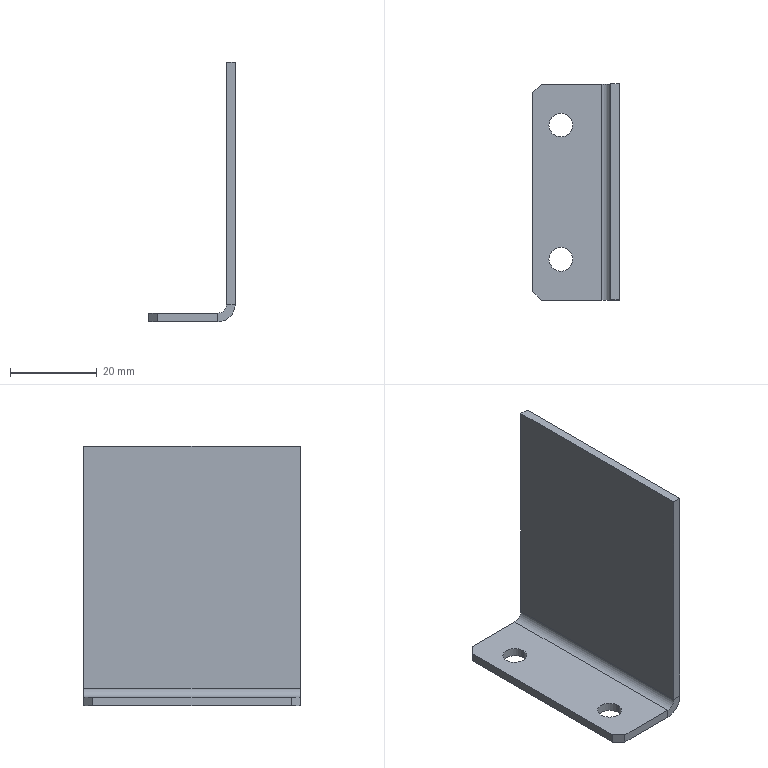Part | STEP file | Cable fixing bracket 1001 | 1 solid | 20 faces | box 20 x 50 x 60 mm | volume 7568 mm3 | plane 14 | cylinder 6 | commonest cylinder face diameters 5.5 x4 4 x1 8 x1
STEP:
#1=CARTESIAN_POINT('',(0.,0.,0.));
#2=DIRECTION('',(0.,0.,1.));
#3=DIRECTION('',(1.,0.,0.));
#4=AXIS2_PLACEMENT_3D('',#1,#2,#3);
#5=CARTESIAN_POINT('',(-16.25,15.5,2.));
#6=VERTEX_POINT('',#5);
#7=CARTESIAN_POINT('',(-16.25,15.5,0.));
#8=VERTEX_POINT('',#7);
#9=CARTESIAN_POINT('',(-16.25,15.5,60.));
#10=DIRECTION('',(0.,0.,-1.));
#11=VECTOR('',#10,1.);
#12=LINE('',#9,#11);
#13=CARTESIAN_POINT('',(-13.5,15.5,60.));
#14=DIRECTION('',(0.,0.,-1.));
#15=DIRECTION('',(-1.,0.,0.));
#16=AXIS2_PLACEMENT_3D('',#13,#14,#15);
#17=CYLINDRICAL_SURFACE('',#16,2.75);
#18=CARTESIAN_POINT('',(6.283,0.));
#19=DIRECTION('',(0.,1.));
#20=VECTOR('',#19,1.);
#21=LINE('',#18,#20);
#22=(GEOMETRIC_REPRESENTATION_CONTEXT(2)PARAMETRIC_REPRESENTATION_CONTEXT()REPRESENTATION_CONTEXT('',''));
#23=DEFINITIONAL_REPRESENTATION('',(#21),#22);
#24=PCURVE('',#17,#23);
#25=CARTESIAN_POINT('',(-13.5,15.5,60.));
#26=DIRECTION('',(0.,0.,-1.));
#27=DIRECTION('',(-1.,0.,0.));
#28=AXIS2_PLACEMENT_3D('',#25,#26,#27);
#29=CYLINDRICAL_SURFACE('',#28,2.75);
#30=CARTESIAN_POINT('',(0.,0.));
#31=DIRECTION('',(0.,1.));
#32=VECTOR('',#31,1.);
#33=LINE('',#30,#32);
#34=(GEOMETRIC_REPRESENTATION_CONTEXT(2)PARAMETRIC_REPRESENTATION_CONTEXT()REPRESENTATION_CONTEXT('',''));
#35=DEFINITIONAL_REPRESENTATION('',(#33),#34);
#36=PCURVE('',#29,#35);
#37=SURFACE_CURVE('',#12,(#24,#36),.PCURVE_S1.);
#38=EDGE_CURVE('',#6,#8,#37,.T.);
#39=ORIENTED_EDGE('',*,*,#38,.T.);
#40=CARTESIAN_POINT('',(-10.75,15.5,0.));
#41=VERTEX_POINT('',#40);
#42=CARTESIAN_POINT('',(-13.5,15.5,0.));
#43=DIRECTION('',(0.,0.,-1.));
#44=DIRECTION('',(-1.,0.,0.));
#45=AXIS2_PLACEMENT_3D('',#42,#43,#44);
#46=CIRCLE('',#45,2.75);
#47=CARTESIAN_POINT('',(0.,60.));
#48=DIRECTION('',(1.,0.));
#49=VECTOR('',#48,1.);
#50=LINE('',#47,#49);
#51=(GEOMETRIC_REPRESENTATION_CONTEXT(2)PARAMETRIC_REPRESENTATION_CONTEXT()REPRESENTATION_CONTEXT('',''));
#52=DEFINITIONAL_REPRESENTATION('',(#50),#51);
#53=PCURVE('',#17,#52);
#54=CARTESIAN_POINT('',(-20.,25.,0.));
#55=DIRECTION('',(0.,0.,-1.));
#56=DIRECTION('',(-1.,0.,0.));
#57=AXIS2_PLACEMENT_3D('',#54,#55,#56);
#58=PLANE('',#57);
#59=CARTESIAN_POINT('',(-6.5,-9.5));
#60=DIRECTION('',(1.,0.));
#61=AXIS2_PLACEMENT_2D('',#59,#60);
#62=CIRCLE('',#61,2.75);
#63=(GEOMETRIC_REPRESENTATION_CONTEXT(2)PARAMETRIC_REPRESENTATION_CONTEXT()REPRESENTATION_CONTEXT('',''));
#64=DEFINITIONAL_REPRESENTATION('',(#62),#63);
#65=PCURVE('',#58,#64);
#66=SURFACE_CURVE('',#46,(#53,#65),.PCURVE_S1.);
#67=EDGE_CURVE('',#41,#8,#66,.T.);
#68=ORIENTED_EDGE('',*,*,#67,.F.);
#69=CARTESIAN_POINT('',(-10.75,15.5,2.));
#70=VERTEX_POINT('',#69);
#71=CARTESIAN_POINT('',(-10.75,15.5,60.));
#72=DIRECTION('',(0.,0.,-1.));
#73=VECTOR('',#72,1.);
#74=LINE('',#71,#73);
#75=CARTESIAN_POINT('',(3.142,0.));
#76=DIRECTION('',(0.,1.));
#77=VECTOR('',#76,1.);
#78=LINE('',#75,#77);
#79=(GEOMETRIC_REPRESENTATION_CONTEXT(2)PARAMETRIC_REPRESENTATION_CONTEXT()REPRESENTATION_CONTEXT('',''));
#80=DEFINITIONAL_REPRESENTATION('',(#78),#79);
#81=PCURVE('',#17,#80);
#82=CARTESIAN_POINT('',(3.142,0.));
#83=DIRECTION('',(0.,1.));
#84=VECTOR('',#83,1.);
#85=LINE('',#82,#84);
#86=(GEOMETRIC_REPRESENTATION_CONTEXT(2)PARAMETRIC_REPRESENTATION_CONTEXT()REPRESENTATION_CONTEXT('',''));
#87=DEFINITIONAL_REPRESENTATION('',(#85),#86);
#88=PCURVE('',#29,#87);
#89=SURFACE_CURVE('',#74,(#81,#88),.PCURVE_S1.);
#90=EDGE_CURVE('',#70,#41,#89,.T.);
#91=ORIENTED_EDGE('',*,*,#90,.F.);
#92=CARTESIAN_POINT('',(-13.5,15.5,2.));
#93=DIRECTION('',(0.,0.,-1.));
#94=DIRECTION('',(-1.,0.,0.));
#95=AXIS2_PLACEMENT_3D('',#92,#93,#94);
#96=CIRCLE('',#95,2.75);
#97=CARTESIAN_POINT('',(0.,58.));
#98=DIRECTION('',(1.,0.));
#99=VECTOR('',#98,1.);
#100=LINE('',#97,#99);
#101=(GEOMETRIC_REPRESENTATION_CONTEXT(2)PARAMETRIC_REPRESENTATION_CONTEXT()REPRESENTATION_CONTEXT('',''));
#102=DEFINITIONAL_REPRESENTATION('',(#100),#101);
#103=PCURVE('',#17,#102);
#104=CARTESIAN_POINT('',(-20.,25.,2.));
#105=DIRECTION('',(0.,0.,-1.));
#106=DIRECTION('',(-1.,0.,0.));
#107=AXIS2_PLACEMENT_3D('',#104,#105,#106);
#108=PLANE('',#107);
#109=CARTESIAN_POINT('',(-6.5,-9.5));
#110=DIRECTION('',(1.,0.));
#111=AXIS2_PLACEMENT_2D('',#109,#110);
#112=CIRCLE('',#111,2.75);
#113=(GEOMETRIC_REPRESENTATION_CONTEXT(2)PARAMETRIC_REPRESENTATION_CONTEXT()REPRESENTATION_CONTEXT('',''));
#114=DEFINITIONAL_REPRESENTATION('',(#112),#113);
#115=PCURVE('',#108,#114);
#116=SURFACE_CURVE('',#96,(#103,#115),.PCURVE_S1.);
#117=EDGE_CURVE('',#70,#6,#116,.T.);
#118=ORIENTED_EDGE('',*,*,#117,.T.);
#119=EDGE_LOOP('',(#39,#68,#91,#118));
#120=FACE_BOUND('',#119,.F.);
#121=ADVANCED_FACE('',(#120),#17,.F.);
#122=CARTESIAN_POINT('',(-16.25,-15.5,2.));
#123=VERTEX_POINT('',#122);
#124=CARTESIAN_POINT('',(-16.25,-15.5,0.));
#125=VERTEX_POINT('',#124);
#126=CARTESIAN_POINT('',(-16.25,-15.5,60.));
#127=DIRECTION('',(0.,0.,-1.));
#128=VECTOR('',#127,1.);
#129=LINE('',#126,#128);
#130=CARTESIAN_POINT('',(-13.5,-15.5,60.));
#131=DIRECTION('',(0.,0.,-1.));
#132=DIRECTION('',(-1.,0.,0.));
#133=AXIS2_PLACEMENT_3D('',#130,#131,#132);
#134=CYLINDRICAL_SURFACE('',#133,2.75);
#135=CARTESIAN_POINT('',(6.283,0.));
#136=DIRECTION('',(0.,1.));
#137=VECTOR('',#136,1.);
#138=LINE('',#135,#137);
#139=(GEOMETRIC_REPRESENTATION_CONTEXT(2)PARAMETRIC_REPRESENTATION_CONTEXT()REPRESENTATION_CONTEXT('',''));
#140=DEFINITIONAL_REPRESENTATION('',(#138),#139);
#141=PCURVE('',#134,#140);
#142=CARTESIAN_POINT('',(-13.5,-15.5,60.));
#143=DIRECTION('',(0.,0.,-1.));
#144=DIRECTION('',(-1.,0.,0.));
#145=AXIS2_PLACEMENT_3D('',#142,#143,#144);
#146=CYLINDRICAL_SURFACE('',#145,2.75);
#147=CARTESIAN_POINT('',(0.,0.));
#148=DIRECTION('',(0.,1.));
#149=VECTOR('',#148,1.);
#150=LINE('',#147,#149);
#151=(GEOMETRIC_REPRESENTATION_CONTEXT(2)PARAMETRIC_REPRESENTATION_CONTEXT()REPRESENTATION_CONTEXT('',''));
#152=DEFINITIONAL_REPRESENTATION('',(#150),#151);
#153=PCURVE('',#146,#152);
#154=SURFACE_CURVE('',#129,(#141,#153),.PCURVE_S1.);
#155=EDGE_CURVE('',#123,#125,#154,.T.);
#156=ORIENTED_EDGE('',*,*,#155,.T.);
#157=CARTESIAN_POINT('',(-10.75,-15.5,0.));
#158=VERTEX_POINT('',#157);
#159=CARTESIAN_POINT('',(-13.5,-15.5,0.));
#160=DIRECTION('',(0.,0.,-1.));
#161=DIRECTION('',(1.,0.,0.));
#162=AXIS2_PLACEMENT_3D('',#159,#160,#161);
#163=CIRCLE('',#162,2.75);
#164=CARTESIAN_POINT('',(3.142,60.));
#165=DIRECTION('',(1.,0.));
#166=VECTOR('',#165,1.);
#167=LINE('',#164,#166);
#168=(GEOMETRIC_REPRESENTATION_CONTEXT(2)PARAMETRIC_REPRESENTATION_CONTEXT()REPRESENTATION_CONTEXT('',''));
#169=DEFINITIONAL_REPRESENTATION('',(#167),#168);
#170=PCURVE('',#134,#169);
#171=CARTESIAN_POINT('',(-6.5,-40.5));
#172=DIRECTION('',(-1.,0.));
#173=AXIS2_PLACEMENT_2D('',#171,#172);
#174=CIRCLE('',#173,2.75);
#175=(GEOMETRIC_REPRESENTATION_CONTEXT(2)PARAMETRIC_REPRESENTATION_CONTEXT()REPRESENTATION_CONTEXT('',''));
#176=DEFINITIONAL_REPRESENTATION('',(#174),#175);
#177=PCURVE('',#58,#176);
#178=SURFACE_CURVE('',#163,(#170,#177),.PCURVE_S1.);
#179=EDGE_CURVE('',#158,#125,#178,.T.);
#180=ORIENTED_EDGE('',*,*,#179,.F.);
#181=CARTESIAN_POINT('',(-10.75,-15.5,2.));
#182=VERTEX_POINT('',#181);
#183=CARTESIAN_POINT('',(-10.75,-15.5,60.));
#184=DIRECTION('',(0.,0.,-1.));
#185=VECTOR('',#184,1.);
#186=LINE('',#183,#185);
#187=CARTESIAN_POINT('',(3.142,0.));
#188=DIRECTION('',(0.,1.));
#189=VECTOR('',#188,1.);
#190=LINE('',#187,#189);
#191=(GEOMETRIC_REPRESENTATION_CONTEXT(2)PARAMETRIC_REPRESENTATION_CONTEXT()REPRESENTATION_CONTEXT('',''));
#192=DEFINITIONAL_REPRESENTATION('',(#190),#191);
#193=PCURVE('',#134,#192);
#194=CARTESIAN_POINT('',(3.142,0.));
#195=DIRECTION('',(0.,1.));
#196=VECTOR('',#195,1.);
#197=LINE('',#194,#196);
#198=(GEOMETRIC_REPRESENTATION_CONTEXT(2)PARAMETRIC_REPRESENTATION_CONTEXT()REPRESENTATION_CONTEXT('',''));
#199=DEFINITIONAL_REPRESENTATION('',(#197),#198);
#200=PCURVE('',#146,#199);
#201=SURFACE_CURVE('',#186,(#193,#200),.PCURVE_S1.);
#202=EDGE_CURVE('',#182,#158,#201,.T.);
#203=ORIENTED_EDGE('',*,*,#202,.F.);
#204=CARTESIAN_POINT('',(-13.5,-15.5,2.));
#205=DIRECTION('',(0.,0.,-1.));
#206=DIRECTION('',(-1.,0.,0.));
#207=AXIS2_PLACEMENT_3D('',#204,#205,#206);
#208=CIRCLE('',#207,2.75);
#209=CARTESIAN_POINT('',(0.,58.));
#210=DIRECTION('',(1.,0.));
#211=VECTOR('',#210,1.);
#212=LINE('',#209,#211);
#213=(GEOMETRIC_REPRESENTATION_CONTEXT(2)PARAMETRIC_REPRESENTATION_CONTEXT()REPRESENTATION_CONTEXT('',''));
#214=DEFINITIONAL_REPRESENTATION('',(#212),#213);
#215=PCURVE('',#134,#214);
#216=CARTESIAN_POINT('',(-6.5,-40.5));
#217=DIRECTION('',(1.,0.));
#218=AXIS2_PLACEMENT_2D('',#216,#217);
#219=CIRCLE('',#218,2.75);
#220=(GEOMETRIC_REPRESENTATION_CONTEXT(2)PARAMETRIC_REPRESENTATION_CONTEXT()REPRESENTATION_CONTEXT('',''));
#221=DEFINITIONAL_REPRESENTATION('',(#219),#220);
#222=PCURVE('',#108,#221);
#223=SURFACE_CURVE('',#208,(#215,#222),.PCURVE_S1.);
#224=EDGE_CURVE('',#182,#123,#223,.T.);
#225=ORIENTED_EDGE('',*,*,#224,.T.);
#226=EDGE_LOOP('',(#156,#180,#203,#225));
#227=FACE_BOUND('',#226,.F.);
#228=ADVANCED_FACE('',(#227),#134,.F.);
#229=CARTESIAN_POINT('',(0.,25.,4.));
#230=VERTEX_POINT('',#229);
#231=CARTESIAN_POINT('',(-2.,25.,4.));
#232=VERTEX_POINT('',#231);
#233=CARTESIAN_POINT('',(0.,25.,4.));
#234=DIRECTION('',(-1.,0.,0.));
#235=VECTOR('',#234,1.);
#236=LINE('',#233,#235);
#237=CARTESIAN_POINT('',(0.,25.,4.));
#238=DIRECTION('',(0.,1.,0.));
#239=DIRECTION('',(0.,0.,1.));
#240=AXIS2_PLACEMENT_3D('',#237,#238,#239);
#241=PLANE('',#240);
#242=CARTESIAN_POINT('',(0.,0.));
#243=DIRECTION('',(0.,-1.));
#244=VECTOR('',#243,1.);
#245=LINE('',#242,#244);
#246=(GEOMETRIC_REPRESENTATION_CONTEXT(2)PARAMETRIC_REPRESENTATION_CONTEXT()REPRESENTATION_CONTEXT('',''));
#247=DEFINITIONAL_REPRESENTATION('',(#245),#246);
#248=PCURVE('',#241,#247);
#249=CARTESIAN_POINT('',(-4.,25.,2.));
#250=DIRECTION('',(0.,1.,0.));
#251=DIRECTION('',(0.,0.,1.));
#252=AXIS2_PLACEMENT_3D('',#249,#250,#251);
#253=PLANE('',#252);
#254=CARTESIAN_POINT('',(2.,4.));
#255=DIRECTION('',(0.,-1.));
#256=VECTOR('',#255,1.);
#257=LINE('',#254,#256);
#258=(GEOMETRIC_REPRESENTATION_CONTEXT(2)PARAMETRIC_REPRESENTATION_CONTEXT()REPRESENTATION_CONTEXT('',''));
#259=DEFINITIONAL_REPRESENTATION('',(#257),#258);
#260=PCURVE('',#253,#259);
#261=SURFACE_CURVE('',#236,(#248,#260),.PCURVE_S1.);
#262=EDGE_CURVE('',#230,#232,#261,.T.);
#263=ORIENTED_EDGE('',*,*,#262,.F.);
#264=CARTESIAN_POINT('',(-4.,25.,0.));
#265=VERTEX_POINT('',#264);
#266=CARTESIAN_POINT('',(-4.,25.,4.));
#267=DIRECTION('',(0.,-1.,0.));
#268=DIRECTION('',(0.,0.,1.));
#269=AXIS2_PLACEMENT_3D('',#266,#267,#268);
#270=CIRCLE('',#269,4.);
#271=CARTESIAN_POINT('',(4.,-4.));
#272=CARTESIAN_POINT('',(4.,-10.928));
#273=CARTESIAN_POINT('',(-2.,-7.464));
#274=CARTESIAN_POINT('',(-8.,-4.));
#275=CARTESIAN_POINT('',(-2.,-0.5359));
#276=CARTESIAN_POINT('',(4.,2.928));
#277=CARTESIAN_POINT('',(4.,-4.));
#278=(BOUNDED_CURVE()B_SPLINE_CURVE(2,(#271,#272,#273,#274,#275,#276,#277),.UNSPECIFIED.,.T.,.F.)B_SPLINE_CURVE_WITH_KNOTS((1,2,2,2,2,1),(-2.094,0.,2.094,4.189,6.283,8.378),.UNSPECIFIED.)CURVE()GEOMETRIC_REPRESENTATION_ITEM()RATIONAL_B_SPLINE_CURVE((1.,0.5,1.,0.5,1.,0.5,1.))REPRESENTATION_ITEM(''));
#279=(GEOMETRIC_REPRESENTATION_CONTEXT(2)PARAMETRIC_REPRESENTATION_CONTEXT()REPRESENTATION_CONTEXT('',''));
#280=DEFINITIONAL_REPRESENTATION('',(#278),#279);
#281=PCURVE('',#241,#280);
#282=CARTESIAN_POINT('',(-4.,25.,4.));
#283=DIRECTION('',(0.,-1.,0.));
#284=DIRECTION('',(0.,0.,-1.));
#285=AXIS2_PLACEMENT_3D('',#282,#283,#284);
#286=CYLINDRICAL_SURFACE('',#285,4.);
#287=CARTESIAN_POINT('',(-3.142,0.));
#288=DIRECTION('',(1.,0.));
#289=VECTOR('',#288,1.);
#290=LINE('',#287,#289);
#291=(GEOMETRIC_REPRESENTATION_CONTEXT(2)PARAMETRIC_REPRESENTATION_CONTEXT()REPRESENTATION_CONTEXT('',''));
#292=DEFINITIONAL_REPRESENTATION('',(#290),#291);
#293=PCURVE('',#286,#292);
#294=SURFACE_CURVE('',#270,(#281,#293),.PCURVE_S1.);
#295=EDGE_CURVE('',#265,#230,#294,.T.);
#296=ORIENTED_EDGE('',*,*,#295,.F.);
#297=CARTESIAN_POINT('',(-4.,25.,2.));
#298=VERTEX_POINT('',#297);
#299=CARTESIAN_POINT('',(-4.,25.,2.));
#300=DIRECTION('',(0.,0.,-1.));
#301=VECTOR('',#300,1.);
#302=LINE('',#299,#301);
#303=CARTESIAN_POINT('',(-2.,-4.));
#304=DIRECTION('',(-1.,0.));
#305=VECTOR('',#304,1.);
#306=LINE('',#303,#305);
#307=(GEOMETRIC_REPRESENTATION_CONTEXT(2)PARAMETRIC_REPRESENTATION_CONTEXT()REPRESENTATION_CONTEXT('',''));
#308=DEFINITIONAL_REPRESENTATION('',(#306),#307);
#309=PCURVE('',#241,#308);
#310=CARTESIAN_POINT('',(-4.,25.,4.));
#311=DIRECTION('',(0.,1.,0.));
#312=DIRECTION('',(1.,0.,0.));
#313=AXIS2_PLACEMENT_3D('',#310,#311,#312);
#314=PLANE('',#313);
#315=CARTESIAN_POINT('',(0.,2.));
#316=DIRECTION('',(0.,1.));
#317=VECTOR('',#316,1.);
#318=LINE('',#315,#317);
#319=(GEOMETRIC_REPRESENTATION_CONTEXT(2)PARAMETRIC_REPRESENTATION_CONTEXT()REPRESENTATION_CONTEXT('',''));
#320=DEFINITIONAL_REPRESENTATION('',(#318),#319);
#321=PCURVE('',#314,#320);
#322=SURFACE_CURVE('',#302,(#309,#321),.PCURVE_S1.);
#323=EDGE_CURVE('',#298,#265,#322,.T.);
#324=ORIENTED_EDGE('',*,*,#323,.F.);
#325=CARTESIAN_POINT('',(-4.,25.,4.));
#326=DIRECTION('',(0.,-1.,0.));
#327=DIRECTION('',(1.,0.,0.));
#328=AXIS2_PLACEMENT_3D('',#325,#326,#327);
#329=CIRCLE('',#328,2.);
#330=CARTESIAN_POINT('',(0.,-2.));
#331=CARTESIAN_POINT('',(3.464,-2.));
#332=CARTESIAN_POINT('',(1.732,-5.));
#333=CARTESIAN_POINT('',(0.,-8.));
#334=CARTESIAN_POINT('',(-1.732,-5.));
#335=CARTESIAN_POINT('',(-3.464,-2.));
#336=CARTESIAN_POINT('',(0.,-2.));
#337=(BOUNDED_CURVE()B_SPLINE_CURVE(2,(#330,#331,#332,#333,#334,#335,#336),.UNSPECIFIED.,.T.,.F.)B_SPLINE_CURVE_WITH_KNOTS((1,2,2,2,2,1),(-2.094,0.,2.094,4.189,6.283,8.378),.UNSPECIFIED.)CURVE()GEOMETRIC_REPRESENTATION_ITEM()RATIONAL_B_SPLINE_CURVE((1.,0.5,1.,0.5,1.,0.5,1.))REPRESENTATION_ITEM(''));
#338=(GEOMETRIC_REPRESENTATION_CONTEXT(2)PARAMETRIC_REPRESENTATION_CONTEXT()REPRESENTATION_CONTEXT('',''));
#339=DEFINITIONAL_REPRESENTATION('',(#337),#338);
#340=PCURVE('',#241,#339);
#341=CARTESIAN_POINT('',(-4.,25.,4.));
#342=DIRECTION('',(0.,-1.,0.));
#343=DIRECTION('',(0.,0.,-1.));
#344=AXIS2_PLACEMENT_3D('',#341,#342,#343);
#345=CYLINDRICAL_SURFACE('',#344,2.);
#346=CARTESIAN_POINT('',(-4.712,0.));
#347=DIRECTION('',(1.,0.));
#348=VECTOR('',#347,1.);
#349=LINE('',#346,#348);
#350=(GEOMETRIC_REPRESENTATION_CONTEXT(2)PARAMETRIC_REPRESENTATION_CONTEXT()REPRESENTATION_CONTEXT('',''));
#351=DEFINITIONAL_REPRESENTATION('',(#349),#350);
#352=PCURVE('',#345,#351);
#353=SURFACE_CURVE('',#329,(#340,#352),.PCURVE_S1.);
#354=EDGE_CURVE('',#298,#232,#353,.T.);
#355=ORIENTED_EDGE('',*,*,#354,.T.);
#356=EDGE_LOOP('',(#263,#296,#324,#355));
#357=FACE_BOUND('',#356,.T.);
#358=ADVANCED_FACE('',(#357),#241,.T.);
#359=CARTESIAN_POINT('',(0.,25.,60.));
#360=VERTEX_POINT('',#359);
#361=CARTESIAN_POINT('',(0.,25.,0.));
#362=DIRECTION('',(0.,0.,1.));
#363=VECTOR('',#362,1.);
#364=LINE('',#361,#363);
#365=CARTESIAN_POINT('',(-2.,4.));
#366=DIRECTION('',(1.,0.));
#367=VECTOR('',#366,1.);
#368=LINE('',#365,#367);
#369=(GEOMETRIC_REPRESENTATION_CONTEXT(2)PARAMETRIC_REPRESENTATION_CONTEXT()REPRESENTATION_CONTEXT('',''));
#370=DEFINITIONAL_REPRESENTATION('',(#368),#369);
#371=PCURVE('',#253,#370);
#372=CARTESIAN_POINT('',(0.,25.,0.));
#373=DIRECTION('',(1.,0.,0.));
#374=DIRECTION('',(0.,0.,-1.));
#375=AXIS2_PLACEMENT_3D('',#372,#373,#374);
#376=PLANE('',#375);
#377=CARTESIAN_POINT('',(0.,0.));
#378=DIRECTION('',(-1.,0.));
#379=VECTOR('',#378,1.);
#380=LINE('',#377,#379);
#381=(GEOMETRIC_REPRESENTATION_CONTEXT(2)PARAMETRIC_REPRESENTATION_CONTEXT()REPRESENTATION_CONTEXT('',''));
#382=DEFINITIONAL_REPRESENTATION('',(#380),#381);
#383=PCURVE('',#376,#382);
#384=SURFACE_CURVE('',#364,(#371,#383),.PCURVE_S1.);
#385=EDGE_CURVE('',#230,#360,#384,.T.);
#386=ORIENTED_EDGE('',*,*,#385,.F.);
#387=ORIENTED_EDGE('',*,*,#262,.T.);
#388=CARTESIAN_POINT('',(-2.,25.,60.));
#389=VERTEX_POINT('',#388);
#390=CARTESIAN_POINT('',(-2.,25.,0.));
#391=DIRECTION('',(0.,0.,1.));
#392=VECTOR('',#391,1.);
#393=LINE('',#390,#392);
#394=CARTESIAN_POINT('',(-2.,2.));
#395=DIRECTION('',(1.,0.));
#396=VECTOR('',#395,1.);
#397=LINE('',#394,#396);
#398=(GEOMETRIC_REPRESENTATION_CONTEXT(2)PARAMETRIC_REPRESENTATION_CONTEXT()REPRESENTATION_CONTEXT('',''));
#399=DEFINITIONAL_REPRESENTATION('',(#397),#398);
#400=PCURVE('',#253,#399);
#401=CARTESIAN_POINT('',(-2.,25.,0.));
#402=DIRECTION('',(1.,0.,0.));
#403=DIRECTION('',(0.,0.,-1.));
#404=AXIS2_PLACEMENT_3D('',#401,#402,#403);
#405=PLANE('',#404);
#406=CARTESIAN_POINT('',(0.,0.));
#407=DIRECTION('',(-1.,0.));
#408=VECTOR('',#407,1.);
#409=LINE('',#406,#408);
#410=(GEOMETRIC_REPRESENTATION_CONTEXT(2)PARAMETRIC_REPRESENTATION_CONTEXT()REPRESENTATION_CONTEXT('',''));
#411=DEFINITIONAL_REPRESENTATION('',(#409),#410);
#412=PCURVE('',#405,#411);
#413=SURFACE_CURVE('',#393,(#400,#412),.PCURVE_S1.);
#414=EDGE_CURVE('',#232,#389,#413,.T.);
#415=ORIENTED_EDGE('',*,*,#414,.T.);
#416=CARTESIAN_POINT('',(0.,25.,60.));
#417=DIRECTION('',(-1.,0.,0.));
#418=VECTOR('',#417,1.);
#419=LINE('',#416,#418);
#420=CARTESIAN_POINT('',(58.,4.));
#421=DIRECTION('',(0.,-1.));
#422=VECTOR('',#421,1.);
#423=LINE('',#420,#422);
#424=(GEOMETRIC_REPRESENTATION_CONTEXT(2)PARAMETRIC_REPRESENTATION_CONTEXT()REPRESENTATION_CONTEXT('',''));
#425=DEFINITIONAL_REPRESENTATION('',(#423),#424);
#426=PCURVE('',#253,#425);
#427=CARTESIAN_POINT('',(0.,25.,60.));
#428=DIRECTION('',(0.,0.,1.));
#429=DIRECTION('',(1.,0.,0.));
#430=AXIS2_PLACEMENT_3D('',#427,#428,#429);
#431=PLANE('',#430);
#432=CARTESIAN_POINT('',(0.,0.));
#433=DIRECTION('',(-1.,0.));
#434=VECTOR('',#433,1.);
#435=LINE('',#432,#434);
#436=(GEOMETRIC_REPRESENTATION_CONTEXT(2)PARAMETRIC_REPRESENTATION_CONTEXT()REPRESENTATION_CONTEXT('',''));
#437=DEFINITIONAL_REPRESENTATION('',(#435),#436);
#438=PCURVE('',#431,#437);
#439=SURFACE_CURVE('',#419,(#426,#438),.PCURVE_S1.);
#440=EDGE_CURVE('',#360,#389,#439,.T.);
#441=ORIENTED_EDGE('',*,*,#440,.F.);
#442=EDGE_LOOP('',(#386,#387,#415,#441));
#443=FACE_BOUND('',#442,.T.);
#444=ADVANCED_FACE('',(#443),#253,.T.);
#445=CARTESIAN_POINT('',(-4.,-25.,0.));
#446=VERTEX_POINT('',#445);
#447=CARTESIAN_POINT('',(-4.,-25.,2.));
#448=VERTEX_POINT('',#447);
#449=CARTESIAN_POINT('',(-4.,-25.,0.));
#450=DIRECTION('',(0.,0.,1.));
#451=VECTOR('',#450,1.);
#452=LINE('',#449,#451);
#453=CARTESIAN_POINT('',(-4.,-25.,0.));
#454=DIRECTION('',(0.,-1.,0.));
#455=DIRECTION('',(0.,0.,-1.));
#456=AXIS2_PLACEMENT_3D('',#453,#454,#455);
#457=PLANE('',#456);
#458=CARTESIAN_POINT('',(0.,0.));
#459=DIRECTION('',(-1.,0.));
#460=VECTOR('',#459,1.);
#461=LINE('',#458,#460);
#462=(GEOMETRIC_REPRESENTATION_CONTEXT(2)PARAMETRIC_REPRESENTATION_CONTEXT()REPRESENTATION_CONTEXT('',''));
#463=DEFINITIONAL_REPRESENTATION('',(#461),#462);
#464=PCURVE('',#457,#463);
#465=CARTESIAN_POINT('',(-2.,-25.,4.));
#466=DIRECTION('',(0.,-1.,0.));
#467=DIRECTION('',(0.,0.,-1.));
#468=AXIS2_PLACEMENT_3D('',#465,#466,#467);
#469=PLANE('',#468);
#470=CARTESIAN_POINT('',(4.,-2.));
#471=DIRECTION('',(-1.,0.));
#472=VECTOR('',#471,1.);
#473=LINE('',#470,#472);
#474=(GEOMETRIC_REPRESENTATION_CONTEXT(2)PARAMETRIC_REPRESENTATION_CONTEXT()REPRESENTATION_CONTEXT('',''));
#475=DEFINITIONAL_REPRESENTATION('',(#473),#474);
#476=PCURVE('',#469,#475);
#477=SURFACE_CURVE('',#452,(#464,#476),.PCURVE_S1.);
#478=EDGE_CURVE('',#446,#448,#477,.T.);
#479=ORIENTED_EDGE('',*,*,#478,.F.);
#480=CARTESIAN_POINT('',(0.,-25.,4.));
#481=VERTEX_POINT('',#480);
#482=CARTESIAN_POINT('',(-4.,-25.,4.));
#483=DIRECTION('',(0.,-1.,0.));
#484=DIRECTION('',(0.,0.,1.));
#485=AXIS2_PLACEMENT_3D('',#482,#483,#484);
#486=CIRCLE('',#485,4.);
#487=CARTESIAN_POINT('',(-4.,0.));
#488=DIRECTION('',(-1.,0.));
#489=AXIS2_PLACEMENT_2D('',#487,#488);
#490=CIRCLE('',#489,4.);
#491=(GEOMETRIC_REPRESENTATION_CONTEXT(2)PARAMETRIC_REPRESENTATION_CONTEXT()REPRESENTATION_CONTEXT('',''));
#492=DEFINITIONAL_REPRESENTATION('',(#490),#491);
#493=PCURVE('',#457,#492);
#494=CARTESIAN_POINT('',(-3.142,50.));
#495=DIRECTION('',(1.,0.));
#496=VECTOR('',#495,1.);
#497=LINE('',#494,#496);
#498=(GEOMETRIC_REPRESENTATION_CONTEXT(2)PARAMETRIC_REPRESENTATION_CONTEXT()REPRESENTATION_CONTEXT('',''));
#499=DEFINITIONAL_REPRESENTATION('',(#497),#498);
#500=PCURVE('',#286,#499);
#501=SURFACE_CURVE('',#486,(#493,#500),.PCURVE_S1.);
#502=EDGE_CURVE('',#446,#481,#501,.T.);
#503=ORIENTED_EDGE('',*,*,#502,.T.);
#504=CARTESIAN_POINT('',(-2.,-25.,4.));
#505=VERTEX_POINT('',#504);
#506=CARTESIAN_POINT('',(-2.,-25.,4.));
#507=DIRECTION('',(1.,0.,0.));
#508=VECTOR('',#507,1.);
#509=LINE('',#506,#508);
#510=CARTESIAN_POINT('',(-4.,2.));
#511=DIRECTION('',(0.,1.));
#512=VECTOR('',#511,1.);
#513=LINE('',#510,#512);
#514=(GEOMETRIC_REPRESENTATION_CONTEXT(2)PARAMETRIC_REPRESENTATION_CONTEXT()REPRESENTATION_CONTEXT('',''));
#515=DEFINITIONAL_REPRESENTATION('',(#513),#514);
#516=PCURVE('',#457,#515);
#517=CARTESIAN_POINT('',(-4.,-25.,4.));
#518=DIRECTION('',(0.,1.,0.));
#519=DIRECTION('',(1.,0.,0.));
#520=AXIS2_PLACEMENT_3D('',#517,#518,#519);
#521=PLANE('',#520);
#522=CARTESIAN_POINT('',(2.,0.));
#523=DIRECTION('',(1.,0.));
#524=VECTOR('',#523,1.);
#525=LINE('',#522,#524);
#526=(GEOMETRIC_REPRESENTATION_CONTEXT(2)PARAMETRIC_REPRESENTATION_CONTEXT()REPRESENTATION_CONTEXT('',''));
#527=DEFINITIONAL_REPRESENTATION('',(#525),#526);
#528=PCURVE('',#521,#527);
#529=SURFACE_CURVE('',#509,(#516,#528),.PCURVE_S1.);
#530=EDGE_CURVE('',#505,#481,#529,.T.);
#531=ORIENTED_EDGE('',*,*,#530,.F.);
#532=CARTESIAN_POINT('',(-4.,-25.,4.));
#533=DIRECTION('',(0.,-1.,0.));
#534=DIRECTION('',(1.,0.,0.));
#535=AXIS2_PLACEMENT_3D('',#532,#533,#534);
#536=CIRCLE('',#535,2.);
#537=CARTESIAN_POINT('',(-4.,0.));
#538=DIRECTION('',(0.,1.));
#539=AXIS2_PLACEMENT_2D('',#537,#538);
#540=CIRCLE('',#539,2.);
#541=(GEOMETRIC_REPRESENTATION_CONTEXT(2)PARAMETRIC_REPRESENTATION_CONTEXT()REPRESENTATION_CONTEXT('',''));
#542=DEFINITIONAL_REPRESENTATION('',(#540),#541);
#543=PCURVE('',#457,#542);
#544=CARTESIAN_POINT('',(-4.712,50.));
#545=DIRECTION('',(1.,0.));
#546=VECTOR('',#545,1.);
#547=LINE('',#544,#546);
#548=(GEOMETRIC_REPRESENTATION_CONTEXT(2)PARAMETRIC_REPRESENTATION_CONTEXT()REPRESENTATION_CONTEXT('',''));
#549=DEFINITIONAL_REPRESENTATION('',(#547),#548);
#550=PCURVE('',#345,#549);
#551=SURFACE_CURVE('',#536,(#543,#550),.PCURVE_S1.);
#552=EDGE_CURVE('',#448,#505,#551,.T.);
#553=ORIENTED_EDGE('',*,*,#552,.F.);
#554=EDGE_LOOP('',(#479,#503,#531,#553));
#555=FACE_BOUND('',#554,.T.);
#556=ADVANCED_FACE('',(#555),#457,.T.);
#557=CARTESIAN_POINT('',(-18.,-25.,2.));
#558=VERTEX_POINT('',#557);
#559=CARTESIAN_POINT('',(-20.,-25.,2.));
#560=DIRECTION('',(1.,0.,0.));
#561=VECTOR('',#560,1.);
#562=LINE('',#559,#561);
#563=CARTESIAN_POINT('',(2.,-18.));
#564=DIRECTION('',(0.,1.));
#565=VECTOR('',#564,1.);
#566=LINE('',#563,#565);
#567=(GEOMETRIC_REPRESENTATION_CONTEXT(2)PARAMETRIC_REPRESENTATION_CONTEXT()REPRESENTATION_CONTEXT('',''));
#568=DEFINITIONAL_REPRESENTATION('',(#566),#567);
#569=PCURVE('',#469,#568);
#570=CARTESIAN_POINT('',(0.,-50.));
#571=DIRECTION('',(-1.,0.));
#572=VECTOR('',#571,1.);
#573=LINE('',#570,#572);
#574=(GEOMETRIC_REPRESENTATION_CONTEXT(2)PARAMETRIC_REPRESENTATION_CONTEXT()REPRESENTATION_CONTEXT('',''));
#575=DEFINITIONAL_REPRESENTATION('',(#573),#574);
#576=PCURVE('',#108,#575);
#577=SURFACE_CURVE('',#562,(#569,#576),.PCURVE_S1.);
#578=EDGE_CURVE('',#558,#448,#577,.T.);
#579=ORIENTED_EDGE('',*,*,#578,.F.);
#580=CARTESIAN_POINT('',(-18.,-25.,0.));
#581=VERTEX_POINT('',#580);
#582=CARTESIAN_POINT('',(-18.,-25.,4.));
#583=DIRECTION('',(0.,0.,-1.));
#584=VECTOR('',#583,1.);
#585=LINE('',#582,#584);
#586=CARTESIAN_POINT('',(0.,-16.));
#587=DIRECTION('',(1.,0.));
#588=VECTOR('',#587,1.);
#589=LINE('',#586,#588);
#590=(GEOMETRIC_REPRESENTATION_CONTEXT(2)PARAMETRIC_REPRESENTATION_CONTEXT()REPRESENTATION_CONTEXT('',''));
#591=DEFINITIONAL_REPRESENTATION('',(#589),#590);
#592=PCURVE('',#469,#591);
#593=CARTESIAN_POINT('',(-18.,-25.,4.));
#594=DIRECTION('',(0.7071,0.7071,0.));
#595=DIRECTION('',(0.,0.,-1.));
#596=AXIS2_PLACEMENT_3D('',#593,#594,#595);
#597=PLANE('',#596);
#598=CARTESIAN_POINT('',(0.,0.));
#599=DIRECTION('',(1.,0.));
#600=VECTOR('',#599,1.);
#601=LINE('',#598,#600);
#602=(GEOMETRIC_REPRESENTATION_CONTEXT(2)PARAMETRIC_REPRESENTATION_CONTEXT()REPRESENTATION_CONTEXT('',''));
#603=DEFINITIONAL_REPRESENTATION('',(#601),#602);
#604=PCURVE('',#597,#603);
#605=SURFACE_CURVE('',#585,(#592,#604),.PCURVE_S1.);
#606=EDGE_CURVE('',#558,#581,#605,.T.);
#607=ORIENTED_EDGE('',*,*,#606,.T.);
#608=CARTESIAN_POINT('',(-20.,-25.,0.));
#609=DIRECTION('',(1.,0.,0.));
#610=VECTOR('',#609,1.);
#611=LINE('',#608,#610);
#612=CARTESIAN_POINT('',(4.,-18.));
#613=DIRECTION('',(0.,1.));
#614=VECTOR('',#613,1.);
#615=LINE('',#612,#614);
#616=(GEOMETRIC_REPRESENTATION_CONTEXT(2)PARAMETRIC_REPRESENTATION_CONTEXT()REPRESENTATION_CONTEXT('',''));
#617=DEFINITIONAL_REPRESENTATION('',(#615),#616);
#618=PCURVE('',#469,#617);
#619=CARTESIAN_POINT('',(0.,-50.));
#620=DIRECTION('',(-1.,0.));
#621=VECTOR('',#620,1.);
#622=LINE('',#619,#621);
#623=(GEOMETRIC_REPRESENTATION_CONTEXT(2)PARAMETRIC_REPRESENTATION_CONTEXT()REPRESENTATION_CONTEXT('',''));
#624=DEFINITIONAL_REPRESENTATION('',(#622),#623);
#625=PCURVE('',#58,#624);
#626=SURFACE_CURVE('',#611,(#618,#625),.PCURVE_S1.);
#627=EDGE_CURVE('',#581,#446,#626,.T.);
#628=ORIENTED_EDGE('',*,*,#627,.T.);
#629=ORIENTED_EDGE('',*,*,#478,.T.);
#630=EDGE_LOOP('',(#579,#607,#628,#629));
#631=FACE_BOUND('',#630,.T.);
#632=ADVANCED_FACE('',(#631),#469,.T.);
#633=CARTESIAN_POINT('',(-2.,-25.,60.));
#634=VERTEX_POINT('',#633);
#635=CARTESIAN_POINT('',(-2.,-25.,0.));
#636=DIRECTION('',(0.,0.,1.));
#637=VECTOR('',#636,1.);
#638=LINE('',#635,#637);
#639=CARTESIAN_POINT('',(0.,-50.));
#640=DIRECTION('',(-1.,0.));
#641=VECTOR('',#640,1.);
#642=LINE('',#639,#641);
#643=(GEOMETRIC_REPRESENTATION_CONTEXT(2)PARAMETRIC_REPRESENTATION_CONTEXT()REPRESENTATION_CONTEXT('',''));
#644=DEFINITIONAL_REPRESENTATION('',(#642),#643);
#645=PCURVE('',#405,#644);
#646=CARTESIAN_POINT('',(2.,4.));
#647=DIRECTION('',(0.,-1.));
#648=VECTOR('',#647,1.);
#649=LINE('',#646,#648);
#650=(GEOMETRIC_REPRESENTATION_CONTEXT(2)PARAMETRIC_REPRESENTATION_CONTEXT()REPRESENTATION_CONTEXT('',''));
#651=DEFINITIONAL_REPRESENTATION('',(#649),#650);
#652=PCURVE('',#521,#651);
#653=SURFACE_CURVE('',#638,(#645,#652),.PCURVE_S1.);
#654=EDGE_CURVE('',#505,#634,#653,.T.);
#655=ORIENTED_EDGE('',*,*,#654,.T.);
#656=CARTESIAN_POINT('',(-2.,25.,60.));
#657=DIRECTION('',(0.,-1.,0.));
#658=VECTOR('',#657,1.);
#659=LINE('',#656,#658);
#660=CARTESIAN_POINT('',(-60.,0.));
#661=DIRECTION('',(0.,-1.));
#662=VECTOR('',#661,1.);
#663=LINE('',#660,#662);
#664=(GEOMETRIC_REPRESENTATION_CONTEXT(2)PARAMETRIC_REPRESENTATION_CONTEXT()REPRESENTATION_CONTEXT('',''));
#665=DEFINITIONAL_REPRESENTATION('',(#663),#664);
#666=PCURVE('',#405,#665);
#667=CARTESIAN_POINT('',(-2.,0.));
#668=DIRECTION('',(0.,-1.));
#669=VECTOR('',#668,1.);
#670=LINE('',#667,#669);
#671=(GEOMETRIC_REPRESENTATION_CONTEXT(2)PARAMETRIC_REPRESENTATION_CONTEXT()REPRESENTATION_CONTEXT('',''));
#672=DEFINITIONAL_REPRESENTATION('',(#670),#671);
#673=PCURVE('',#431,#672);
#674=SURFACE_CURVE('',#659,(#666,#673),.PCURVE_S1.);
#675=EDGE_CURVE('',#389,#634,#674,.T.);
#676=ORIENTED_EDGE('',*,*,#675,.F.);
#677=ORIENTED_EDGE('',*,*,#414,.F.);
#678=CARTESIAN_POINT('',(-2.,25.,4.));
#679=DIRECTION('',(0.,-1.,0.));
#680=VECTOR('',#679,1.);
#681=LINE('',#678,#680);
#682=CARTESIAN_POINT('',(-4.,0.));
#683=DIRECTION('',(0.,-1.));
#684=VECTOR('',#683,1.);
#685=LINE('',#682,#684);
#686=(GEOMETRIC_REPRESENTATION_CONTEXT(2)PARAMETRIC_REPRESENTATION_CONTEXT()REPRESENTATION_CONTEXT('',''));
#687=DEFINITIONAL_REPRESENTATION('',(#685),#686);
#688=PCURVE('',#405,#687);
#689=CARTESIAN_POINT('',(1.571,0.));
#690=DIRECTION('',(0.,1.));
#691=VECTOR('',#690,1.);
#692=LINE('',#689,#691);
#693=(GEOMETRIC_REPRESENTATION_CONTEXT(2)PARAMETRIC_REPRESENTATION_CONTEXT()REPRESENTATION_CONTEXT('',''));
#694=DEFINITIONAL_REPRESENTATION('',(#692),#693);
#695=PCURVE('',#345,#694);
#696=SURFACE_CURVE('',#681,(#688,#695),.PCURVE_S1.);
#697=EDGE_CURVE('',#232,#505,#696,.T.);
#698=ORIENTED_EDGE('',*,*,#697,.T.);
#699=EDGE_LOOP('',(#655,#676,#677,#698));
#700=FACE_BOUND('',#699,.T.);
#701=ADVANCED_FACE('',(#700),#405,.F.);
#702=CARTESIAN_POINT('',(0.,-25.,60.));
#703=VERTEX_POINT('',#702);
#704=CARTESIAN_POINT('',(0.,-25.,60.));
#705=DIRECTION('',(-1.,0.,0.));
#706=VECTOR('',#705,1.);
#707=LINE('',#704,#706);
#708=CARTESIAN_POINT('',(0.,-50.));
#709=DIRECTION('',(-1.,0.));
#710=VECTOR('',#709,1.);
#711=LINE('',#708,#710);
#712=(GEOMETRIC_REPRESENTATION_CONTEXT(2)PARAMETRIC_REPRESENTATION_CONTEXT()REPRESENTATION_CONTEXT('',''));
#713=DEFINITIONAL_REPRESENTATION('',(#711),#712);
#714=PCURVE('',#431,#713);
#715=CARTESIAN_POINT('',(4.,-56.));
#716=DIRECTION('',(-1.,0.));
#717=VECTOR('',#716,1.);
#718=LINE('',#715,#717);
#719=(GEOMETRIC_REPRESENTATION_CONTEXT(2)PARAMETRIC_REPRESENTATION_CONTEXT()REPRESENTATION_CONTEXT('',''));
#720=DEFINITIONAL_REPRESENTATION('',(#718),#719);
#721=PCURVE('',#521,#720);
#722=SURFACE_CURVE('',#707,(#714,#721),.PCURVE_S1.);
#723=EDGE_CURVE('',#703,#634,#722,.T.);
#724=ORIENTED_EDGE('',*,*,#723,.F.);
#725=CARTESIAN_POINT('',(0.,25.,60.));
#726=DIRECTION('',(0.,-1.,0.));
#727=VECTOR('',#726,1.);
#728=LINE('',#725,#727);
#729=CARTESIAN_POINT('',(0.,0.));
#730=DIRECTION('',(0.,-1.));
#731=VECTOR('',#730,1.);
#732=LINE('',#729,#731);
#733=(GEOMETRIC_REPRESENTATION_CONTEXT(2)PARAMETRIC_REPRESENTATION_CONTEXT()REPRESENTATION_CONTEXT('',''));
#734=DEFINITIONAL_REPRESENTATION('',(#732),#733);
#735=PCURVE('',#431,#734);
#736=CARTESIAN_POINT('',(-60.,0.));
#737=DIRECTION('',(0.,-1.));
#738=VECTOR('',#737,1.);
#739=LINE('',#736,#738);
#740=(GEOMETRIC_REPRESENTATION_CONTEXT(2)PARAMETRIC_REPRESENTATION_CONTEXT()REPRESENTATION_CONTEXT('',''));
#741=DEFINITIONAL_REPRESENTATION('',(#739),#740);
#742=PCURVE('',#376,#741);
#743=SURFACE_CURVE('',#728,(#735,#742),.PCURVE_S1.);
#744=EDGE_CURVE('',#360,#703,#743,.T.);
#745=ORIENTED_EDGE('',*,*,#744,.F.);
#746=ORIENTED_EDGE('',*,*,#440,.T.);
#747=ORIENTED_EDGE('',*,*,#675,.T.);
#748=EDGE_LOOP('',(#724,#745,#746,#747));
#749=FACE_BOUND('',#748,.T.);
#750=ADVANCED_FACE('',(#749),#431,.T.);
#751=CARTESIAN_POINT('',(0.,-25.,0.));
#752=DIRECTION('',(0.,0.,1.));
#753=VECTOR('',#752,1.);
#754=LINE('',#751,#753);
#755=CARTESIAN_POINT('',(0.,-50.));
#756=DIRECTION('',(-1.,0.));
#757=VECTOR('',#756,1.);
#758=LINE('',#755,#757);
#759=(GEOMETRIC_REPRESENTATION_CONTEXT(2)PARAMETRIC_REPRESENTATION_CONTEXT()REPRESENTATION_CONTEXT('',''));
#760=DEFINITIONAL_REPRESENTATION('',(#758),#759);
#761=PCURVE('',#376,#760);
#762=CARTESIAN_POINT('',(4.,4.));
#763=DIRECTION('',(0.,-1.));
#764=VECTOR('',#763,1.);
#765=LINE('',#762,#764);
#766=(GEOMETRIC_REPRESENTATION_CONTEXT(2)PARAMETRIC_REPRESENTATION_CONTEXT()REPRESENTATION_CONTEXT('',''));
#767=DEFINITIONAL_REPRESENTATION('',(#765),#766);
#768=PCURVE('',#521,#767);
#769=SURFACE_CURVE('',#754,(#761,#768),.PCURVE_S1.);
#770=EDGE_CURVE('',#481,#703,#769,.T.);
#771=ORIENTED_EDGE('',*,*,#770,.F.);
#772=CARTESIAN_POINT('',(0.,25.,4.));
#773=DIRECTION('',(0.,-1.,0.));
#774=VECTOR('',#773,1.);
#775=LINE('',#772,#774);
#776=CARTESIAN_POINT('',(-4.,0.));
#777=DIRECTION('',(0.,-1.));
#778=VECTOR('',#777,1.);
#779=LINE('',#776,#778);
#780=(GEOMETRIC_REPRESENTATION_CONTEXT(2)PARAMETRIC_REPRESENTATION_CONTEXT()REPRESENTATION_CONTEXT('',''));
#781=DEFINITIONAL_REPRESENTATION('',(#779),#780);
#782=PCURVE('',#376,#781);
#783=CARTESIAN_POINT('',(1.571,0.));
#784=DIRECTION('',(0.,1.));
#785=VECTOR('',#784,1.);
#786=LINE('',#783,#785);
#787=(GEOMETRIC_REPRESENTATION_CONTEXT(2)PARAMETRIC_REPRESENTATION_CONTEXT()REPRESENTATION_CONTEXT('',''));
#788=DEFINITIONAL_REPRESENTATION('',(#786),#787);
#789=PCURVE('',#286,#788);
#790=SURFACE_CURVE('',#775,(#782,#789),.PCURVE_S1.);
#791=EDGE_CURVE('',#230,#481,#790,.T.);
#792=ORIENTED_EDGE('',*,*,#791,.F.);
#793=ORIENTED_EDGE('',*,*,#385,.T.);
#794=ORIENTED_EDGE('',*,*,#744,.T.);
#795=EDGE_LOOP('',(#771,#792,#793,#794));
#796=FACE_BOUND('',#795,.T.);
#797=ADVANCED_FACE('',(#796),#376,.T.);
#798=ORIENTED_EDGE('',*,*,#502,.F.);
#799=CARTESIAN_POINT('',(-4.,25.,0.));
#800=DIRECTION('',(0.,-1.,0.));
#801=VECTOR('',#800,1.);
#802=LINE('',#799,#801);
#803=CARTESIAN_POINT('',(0.,0.));
#804=DIRECTION('',(0.,1.));
#805=VECTOR('',#804,1.);
#806=LINE('',#803,#805);
#807=(GEOMETRIC_REPRESENTATION_CONTEXT(2)PARAMETRIC_REPRESENTATION_CONTEXT()REPRESENTATION_CONTEXT('',''));
#808=DEFINITIONAL_REPRESENTATION('',(#806),#807);
#809=PCURVE('',#286,#808);
#810=CARTESIAN_POINT('',(-16.,0.));
#811=DIRECTION('',(0.,-1.));
#812=VECTOR('',#811,1.);
#813=LINE('',#810,#812);
#814=(GEOMETRIC_REPRESENTATION_CONTEXT(2)PARAMETRIC_REPRESENTATION_CONTEXT()REPRESENTATION_CONTEXT('',''));
#815=DEFINITIONAL_REPRESENTATION('',(#813),#814);
#816=PCURVE('',#58,#815);
#817=SURFACE_CURVE('',#802,(#809,#816),.PCURVE_S1.);
#818=EDGE_CURVE('',#265,#446,#817,.T.);
#819=ORIENTED_EDGE('',*,*,#818,.F.);
#820=ORIENTED_EDGE('',*,*,#295,.T.);
#821=ORIENTED_EDGE('',*,*,#791,.T.);
#822=EDGE_LOOP('',(#798,#819,#820,#821));
#823=FACE_BOUND('',#822,.T.);
#824=ADVANCED_FACE('',(#823),#286,.T.);
#825=CARTESIAN_POINT('',(-13.5,15.5,0.));
#826=DIRECTION('',(0.,0.,-1.));
#827=DIRECTION('',(-1.,0.,0.));
#828=AXIS2_PLACEMENT_3D('',#825,#826,#827);
#829=CIRCLE('',#828,2.75);
#830=CARTESIAN_POINT('',(-6.5,-9.5));
#831=DIRECTION('',(1.,0.));
#832=AXIS2_PLACEMENT_2D('',#830,#831);
#833=CIRCLE('',#832,2.75);
#834=(GEOMETRIC_REPRESENTATION_CONTEXT(2)PARAMETRIC_REPRESENTATION_CONTEXT()REPRESENTATION_CONTEXT('',''));
#835=DEFINITIONAL_REPRESENTATION('',(#833),#834);
#836=PCURVE('',#58,#835);
#837=CARTESIAN_POINT('',(0.,60.));
#838=DIRECTION('',(1.,0.));
#839=VECTOR('',#838,1.);
#840=LINE('',#837,#839);
#841=(GEOMETRIC_REPRESENTATION_CONTEXT(2)PARAMETRIC_REPRESENTATION_CONTEXT()REPRESENTATION_CONTEXT('',''));
#842=DEFINITIONAL_REPRESENTATION('',(#840),#841);
#843=PCURVE('',#29,#842);
#844=SURFACE_CURVE('',#829,(#836,#843),.PCURVE_S1.);
#845=EDGE_CURVE('',#8,#41,#844,.T.);
#846=ORIENTED_EDGE('',*,*,#845,.F.);
#847=ORIENTED_EDGE('',*,*,#67,.F.);
#848=EDGE_LOOP('',(#846,#847));
#849=FACE_BOUND('',#848,.T.);
#850=CARTESIAN_POINT('',(-13.5,-15.5,0.));
#851=DIRECTION('',(0.,0.,-1.));
#852=DIRECTION('',(1.,0.,0.));
#853=AXIS2_PLACEMENT_3D('',#850,#851,#852);
#854=CIRCLE('',#853,2.75);
#855=CARTESIAN_POINT('',(-6.5,-40.5));
#856=DIRECTION('',(-1.,0.));
#857=AXIS2_PLACEMENT_2D('',#855,#856);
#858=CIRCLE('',#857,2.75);
#859=(GEOMETRIC_REPRESENTATION_CONTEXT(2)PARAMETRIC_REPRESENTATION_CONTEXT()REPRESENTATION_CONTEXT('',''));
#860=DEFINITIONAL_REPRESENTATION('',(#858),#859);
#861=PCURVE('',#58,#860);
#862=CARTESIAN_POINT('',(-3.142,60.));
#863=DIRECTION('',(1.,0.));
#864=VECTOR('',#863,1.);
#865=LINE('',#862,#864);
#866=(GEOMETRIC_REPRESENTATION_CONTEXT(2)PARAMETRIC_REPRESENTATION_CONTEXT()REPRESENTATION_CONTEXT('',''));
#867=DEFINITIONAL_REPRESENTATION('',(#865),#866);
#868=PCURVE('',#146,#867);
#869=SURFACE_CURVE('',#854,(#861,#868),.PCURVE_S1.);
#870=EDGE_CURVE('',#125,#158,#869,.T.);
#871=ORIENTED_EDGE('',*,*,#870,.F.);
#872=ORIENTED_EDGE('',*,*,#179,.F.);
#873=EDGE_LOOP('',(#871,#872));
#874=FACE_BOUND('',#873,.T.);
#875=ORIENTED_EDGE('',*,*,#627,.F.);
#876=CARTESIAN_POINT('',(-20.,-23.,0.));
#877=VERTEX_POINT('',#876);
#878=CARTESIAN_POINT('',(-44.,1.,0.));
#879=DIRECTION('',(-0.7071,0.7071,0.));
#880=VECTOR('',#879,1.);
#881=LINE('',#878,#880);
#882=CARTESIAN_POINT('',(24.,-24.));
#883=DIRECTION('',(0.7071,0.7071));
#884=VECTOR('',#883,1.);
#885=LINE('',#882,#884);
#886=(GEOMETRIC_REPRESENTATION_CONTEXT(2)PARAMETRIC_REPRESENTATION_CONTEXT()REPRESENTATION_CONTEXT('',''));
#887=DEFINITIONAL_REPRESENTATION('',(#885),#886);
#888=PCURVE('',#58,#887);
#889=CARTESIAN_POINT('',(4.,36.77));
#890=DIRECTION('',(0.,1.));
#891=VECTOR('',#890,1.);
#892=LINE('',#889,#891);
#893=(GEOMETRIC_REPRESENTATION_CONTEXT(2)PARAMETRIC_REPRESENTATION_CONTEXT()REPRESENTATION_CONTEXT('',''));
#894=DEFINITIONAL_REPRESENTATION('',(#892),#893);
#895=PCURVE('',#597,#894);
#896=SURFACE_CURVE('',#881,(#888,#895),.PCURVE_S1.);
#897=EDGE_CURVE('',#581,#877,#896,.T.);
#898=ORIENTED_EDGE('',*,*,#897,.T.);
#899=CARTESIAN_POINT('',(-20.,23.,0.));
#900=VERTEX_POINT('',#899);
#901=CARTESIAN_POINT('',(-20.,25.,0.));
#902=DIRECTION('',(0.,-1.,0.));
#903=VECTOR('',#902,1.);
#904=LINE('',#901,#903);
#905=CARTESIAN_POINT('',(0.,0.));
#906=DIRECTION('',(0.,-1.));
#907=VECTOR('',#906,1.);
#908=LINE('',#905,#907);
#909=(GEOMETRIC_REPRESENTATION_CONTEXT(2)PARAMETRIC_REPRESENTATION_CONTEXT()REPRESENTATION_CONTEXT('',''));
#910=DEFINITIONAL_REPRESENTATION('',(#908),#909);
#911=PCURVE('',#58,#910);
#912=CARTESIAN_POINT('',(-20.,25.,2.));
#913=DIRECTION('',(-1.,0.,0.));
#914=DIRECTION('',(0.,0.,1.));
#915=AXIS2_PLACEMENT_3D('',#912,#913,#914);
#916=PLANE('',#915);
#917=CARTESIAN_POINT('',(-2.,0.));
#918=DIRECTION('',(0.,-1.));
#919=VECTOR('',#918,1.);
#920=LINE('',#917,#919);
#921=(GEOMETRIC_REPRESENTATION_CONTEXT(2)PARAMETRIC_REPRESENTATION_CONTEXT()REPRESENTATION_CONTEXT('',''));
#922=DEFINITIONAL_REPRESENTATION('',(#920),#921);
#923=PCURVE('',#916,#922);
#924=SURFACE_CURVE('',#904,(#911,#923),.PCURVE_S1.);
#925=EDGE_CURVE('',#900,#877,#924,.T.);
#926=ORIENTED_EDGE('',*,*,#925,.F.);
#927=CARTESIAN_POINT('',(-18.,25.,0.));
#928=VERTEX_POINT('',#927);
#929=CARTESIAN_POINT('',(-19.,24.,0.));
#930=DIRECTION('',(0.7071,0.7071,0.));
#931=VECTOR('',#930,1.);
#932=LINE('',#929,#931);
#933=CARTESIAN_POINT('',(-1.,-1.));
#934=DIRECTION('',(-0.7071,0.7071));
#935=VECTOR('',#934,1.);
#936=LINE('',#933,#935);
#937=(GEOMETRIC_REPRESENTATION_CONTEXT(2)PARAMETRIC_REPRESENTATION_CONTEXT()REPRESENTATION_CONTEXT('',''));
#938=DEFINITIONAL_REPRESENTATION('',(#936),#937);
#939=PCURVE('',#58,#938);
#940=CARTESIAN_POINT('',(-20.,23.,2.));
#941=DIRECTION('',(0.7071,-0.7071,0.));
#942=DIRECTION('',(0.,0.,-1.));
#943=AXIS2_PLACEMENT_3D('',#940,#941,#942);
#944=PLANE('',#943);
#945=CARTESIAN_POINT('',(2.,1.414));
#946=DIRECTION('',(0.,1.));
#947=VECTOR('',#946,1.);
#948=LINE('',#945,#947);
#949=(GEOMETRIC_REPRESENTATION_CONTEXT(2)PARAMETRIC_REPRESENTATION_CONTEXT()REPRESENTATION_CONTEXT('',''));
#950=DEFINITIONAL_REPRESENTATION('',(#948),#949);
#951=PCURVE('',#944,#950);
#952=SURFACE_CURVE('',#932,(#939,#951),.PCURVE_S1.);
#953=EDGE_CURVE('',#900,#928,#952,.T.);
#954=ORIENTED_EDGE('',*,*,#953,.T.);
#955=CARTESIAN_POINT('',(-20.,25.,0.));
#956=DIRECTION('',(1.,0.,0.));
#957=VECTOR('',#956,1.);
#958=LINE('',#955,#957);
#959=CARTESIAN_POINT('',(0.,0.));
#960=DIRECTION('',(-1.,0.));
#961=VECTOR('',#960,1.);
#962=LINE('',#959,#961);
#963=(GEOMETRIC_REPRESENTATION_CONTEXT(2)PARAMETRIC_REPRESENTATION_CONTEXT()REPRESENTATION_CONTEXT('',''));
#964=DEFINITIONAL_REPRESENTATION('',(#962),#963);
#965=PCURVE('',#58,#964);
#966=CARTESIAN_POINT('',(-16.,4.));
#967=DIRECTION('',(1.,0.));
#968=VECTOR('',#967,1.);
#969=LINE('',#966,#968);
#970=(GEOMETRIC_REPRESENTATION_CONTEXT(2)PARAMETRIC_REPRESENTATION_CONTEXT()REPRESENTATION_CONTEXT('',''));
#971=DEFINITIONAL_REPRESENTATION('',(#969),#970);
#972=PCURVE('',#314,#971);
#973=SURFACE_CURVE('',#958,(#965,#972),.PCURVE_S1.);
#974=EDGE_CURVE('',#928,#265,#973,.T.);
#975=ORIENTED_EDGE('',*,*,#974,.T.);
#976=ORIENTED_EDGE('',*,*,#818,.T.);
#977=EDGE_LOOP('',(#875,#898,#926,#954,#975,#976));
#978=FACE_BOUND('',#977,.T.);
#979=ADVANCED_FACE('',(#849,#874,#978),#58,.T.);
#980=ORIENTED_EDGE('',*,*,#925,.T.);
#981=CARTESIAN_POINT('',(-20.,-23.,2.));
#982=VERTEX_POINT('',#981);
#983=CARTESIAN_POINT('',(-20.,-23.,2.));
#984=DIRECTION('',(0.,0.,1.));
#985=VECTOR('',#984,1.);
#986=LINE('',#983,#985);
#987=CARTESIAN_POINT('',(0.,-48.));
#988=DIRECTION('',(1.,0.));
#989=VECTOR('',#988,1.);
#990=LINE('',#987,#989);
#991=(GEOMETRIC_REPRESENTATION_CONTEXT(2)PARAMETRIC_REPRESENTATION_CONTEXT()REPRESENTATION_CONTEXT('',''));
#992=DEFINITIONAL_REPRESENTATION('',(#990),#991);
#993=PCURVE('',#916,#992);
#994=CARTESIAN_POINT('',(2.,2.828));
#995=DIRECTION('',(-1.,0.));
#996=VECTOR('',#995,1.);
#997=LINE('',#994,#996);
#998=(GEOMETRIC_REPRESENTATION_CONTEXT(2)PARAMETRIC_REPRESENTATION_CONTEXT()REPRESENTATION_CONTEXT('',''));
#999=DEFINITIONAL_REPRESENTATION('',(#997),#998);
#1000=PCURVE('',#597,#999);
#1001=SURFACE_CURVE('',#986,(#993,#1000),.PCURVE_S1.);
#1002=EDGE_CURVE('',#877,#982,#1001,.T.);
#1003=ORIENTED_EDGE('',*,*,#1002,.T.);
#1004=CARTESIAN_POINT('',(-20.,23.,2.));
#1005=VERTEX_POINT('',#1004);
#1006=CARTESIAN_POINT('',(-20.,25.,2.));
#1007=DIRECTION('',(0.,-1.,0.));
#1008=VECTOR('',#1007,1.);
#1009=LINE('',#1006,#1008);
#1010=CARTESIAN_POINT('',(0.,0.));
#1011=DIRECTION('',(0.,-1.));
#1012=VECTOR('',#1011,1.);
#1013=LINE('',#1010,#1012);
#1014=(GEOMETRIC_REPRESENTATION_CONTEXT(2)PARAMETRIC_REPRESENTATION_CONTEXT()REPRESENTATION_CONTEXT('',''));
#1015=DEFINITIONAL_REPRESENTATION('',(#1013),#1014);
#1016=PCURVE('',#916,#1015);
#1017=CARTESIAN_POINT('',(0.,0.));
#1018=DIRECTION('',(0.,-1.));
#1019=VECTOR('',#1018,1.);
#1020=LINE('',#1017,#1019);
#1021=(GEOMETRIC_REPRESENTATION_CONTEXT(2)PARAMETRIC_REPRESENTATION_CONTEXT()REPRESENTATION_CONTEXT('',''));
#1022=DEFINITIONAL_REPRESENTATION('',(#1020),#1021);
#1023=PCURVE('',#108,#1022);
#1024=SURFACE_CURVE('',#1009,(#1016,#1023),.PCURVE_S1.);
#1025=EDGE_CURVE('',#1005,#982,#1024,.T.);
#1026=ORIENTED_EDGE('',*,*,#1025,.F.);
#1027=CARTESIAN_POINT('',(-20.,23.,2.));
#1028=DIRECTION('',(0.,0.,-1.));
#1029=VECTOR('',#1028,1.);
#1030=LINE('',#1027,#1029);
#1031=CARTESIAN_POINT('',(0.,-2.));
#1032=DIRECTION('',(-1.,0.));
#1033=VECTOR('',#1032,1.);
#1034=LINE('',#1031,#1033);
#1035=(GEOMETRIC_REPRESENTATION_CONTEXT(2)PARAMETRIC_REPRESENTATION_CONTEXT()REPRESENTATION_CONTEXT('',''));
#1036=DEFINITIONAL_REPRESENTATION('',(#1034),#1035);
#1037=PCURVE('',#916,#1036);
#1038=CARTESIAN_POINT('',(0.,0.));
#1039=DIRECTION('',(1.,0.));
#1040=VECTOR('',#1039,1.);
#1041=LINE('',#1038,#1040);
#1042=(GEOMETRIC_REPRESENTATION_CONTEXT(2)PARAMETRIC_REPRESENTATION_CONTEXT()REPRESENTATION_CONTEXT('',''));
#1043=DEFINITIONAL_REPRESENTATION('',(#1041),#1042);
#1044=PCURVE('',#944,#1043);
#1045=SURFACE_CURVE('',#1030,(#1037,#1044),.PCURVE_S1.);
#1046=EDGE_CURVE('',#1005,#900,#1045,.T.);
#1047=ORIENTED_EDGE('',*,*,#1046,.T.);
#1048=EDGE_LOOP('',(#980,#1003,#1026,#1047));
#1049=FACE_BOUND('',#1048,.T.);
#1050=ADVANCED_FACE('',(#1049),#916,.T.);
#1051=CARTESIAN_POINT('',(-13.5,15.5,2.));
#1052=DIRECTION('',(0.,0.,-1.));
#1053=DIRECTION('',(-1.,0.,0.));
#1054=AXIS2_PLACEMENT_3D('',#1051,#1052,#1053);
#1055=CIRCLE('',#1054,2.75);
#1056=CARTESIAN_POINT('',(-6.5,-9.5));
#1057=DIRECTION('',(1.,0.));
#1058=AXIS2_PLACEMENT_2D('',#1056,#1057);
#1059=CIRCLE('',#1058,2.75);
#1060=(GEOMETRIC_REPRESENTATION_CONTEXT(2)PARAMETRIC_REPRESENTATION_CONTEXT()REPRESENTATION_CONTEXT('',''));
#1061=DEFINITIONAL_REPRESENTATION('',(#1059),#1060);
#1062=PCURVE('',#108,#1061);
#1063=CARTESIAN_POINT('',(0.,58.));
#1064=DIRECTION('',(1.,0.));
#1065=VECTOR('',#1064,1.);
#1066=LINE('',#1063,#1065);
#1067=(GEOMETRIC_REPRESENTATION_CONTEXT(2)PARAMETRIC_REPRESENTATION_CONTEXT()REPRESENTATION_CONTEXT('',''));
#1068=DEFINITIONAL_REPRESENTATION('',(#1066),#1067);
#1069=PCURVE('',#29,#1068);
#1070=SURFACE_CURVE('',#1055,(#1062,#1069),.PCURVE_S1.);
#1071=EDGE_CURVE('',#6,#70,#1070,.T.);
#1072=ORIENTED_EDGE('',*,*,#1071,.T.);
#1073=ORIENTED_EDGE('',*,*,#117,.T.);
#1074=EDGE_LOOP('',(#1072,#1073));
#1075=FACE_BOUND('',#1074,.T.);
#1076=CARTESIAN_POINT('',(-13.5,-15.5,2.));
#1077=DIRECTION('',(0.,0.,-1.));
#1078=DIRECTION('',(-1.,0.,0.));
#1079=AXIS2_PLACEMENT_3D('',#1076,#1077,#1078);
#1080=CIRCLE('',#1079,2.75);
#1081=CARTESIAN_POINT('',(-6.5,-40.5));
#1082=DIRECTION('',(1.,0.));
#1083=AXIS2_PLACEMENT_2D('',#1081,#1082);
#1084=CIRCLE('',#1083,2.75);
#1085=(GEOMETRIC_REPRESENTATION_CONTEXT(2)PARAMETRIC_REPRESENTATION_CONTEXT()REPRESENTATION_CONTEXT('',''));
#1086=DEFINITIONAL_REPRESENTATION('',(#1084),#1085);
#1087=PCURVE('',#108,#1086);
#1088=CARTESIAN_POINT('',(0.,58.));
#1089=DIRECTION('',(1.,0.));
#1090=VECTOR('',#1089,1.);
#1091=LINE('',#1088,#1090);
#1092=(GEOMETRIC_REPRESENTATION_CONTEXT(2)PARAMETRIC_REPRESENTATION_CONTEXT()REPRESENTATION_CONTEXT('',''));
#1093=DEFINITIONAL_REPRESENTATION('',(#1091),#1092);
#1094=PCURVE('',#146,#1093);
#1095=SURFACE_CURVE('',#1080,(#1087,#1094),.PCURVE_S1.);
#1096=EDGE_CURVE('',#123,#182,#1095,.T.);
#1097=ORIENTED_EDGE('',*,*,#1096,.T.);
#1098=ORIENTED_EDGE('',*,*,#224,.T.);
#1099=EDGE_LOOP('',(#1097,#1098));
#1100=FACE_BOUND('',#1099,.T.);
#1101=ORIENTED_EDGE('',*,*,#1025,.T.);
#1102=CARTESIAN_POINT('',(-18.,-25.,2.));
#1103=DIRECTION('',(0.7071,-0.7071,0.));
#1104=VECTOR('',#1103,1.);
#1105=LINE('',#1102,#1104);
#1106=CARTESIAN_POINT('',(-2.,-50.));
#1107=DIRECTION('',(-0.7071,-0.7071));
#1108=VECTOR('',#1107,1.);
#1109=LINE('',#1106,#1108);
#1110=(GEOMETRIC_REPRESENTATION_CONTEXT(2)PARAMETRIC_REPRESENTATION_CONTEXT()REPRESENTATION_CONTEXT('',''));
#1111=DEFINITIONAL_REPRESENTATION('',(#1109),#1110);
#1112=PCURVE('',#108,#1111);
#1113=CARTESIAN_POINT('',(2.,0.));
#1114=DIRECTION('',(0.,-1.));
#1115=VECTOR('',#1114,1.);
#1116=LINE('',#1113,#1115);
#1117=(GEOMETRIC_REPRESENTATION_CONTEXT(2)PARAMETRIC_REPRESENTATION_CONTEXT()REPRESENTATION_CONTEXT('',''));
#1118=DEFINITIONAL_REPRESENTATION('',(#1116),#1117);
#1119=PCURVE('',#597,#1118);
#1120=SURFACE_CURVE('',#1105,(#1112,#1119),.PCURVE_S1.);
#1121=EDGE_CURVE('',#982,#558,#1120,.T.);
#1122=ORIENTED_EDGE('',*,*,#1121,.T.);
#1123=ORIENTED_EDGE('',*,*,#578,.T.);
#1124=CARTESIAN_POINT('',(-4.,25.,2.));
#1125=DIRECTION('',(0.,-1.,0.));
#1126=VECTOR('',#1125,1.);
#1127=LINE('',#1124,#1126);
#1128=CARTESIAN_POINT('',(-16.,0.));
#1129=DIRECTION('',(0.,-1.));
#1130=VECTOR('',#1129,1.);
#1131=LINE('',#1128,#1130);
#1132=(GEOMETRIC_REPRESENTATION_CONTEXT(2)PARAMETRIC_REPRESENTATION_CONTEXT()REPRESENTATION_CONTEXT('',''));
#1133=DEFINITIONAL_REPRESENTATION('',(#1131),#1132);
#1134=PCURVE('',#108,#1133);
#1135=CARTESIAN_POINT('',(0.,0.));
#1136=DIRECTION('',(0.,1.));
#1137=VECTOR('',#1136,1.);
#1138=LINE('',#1135,#1137);
#1139=(GEOMETRIC_REPRESENTATION_CONTEXT(2)PARAMETRIC_REPRESENTATION_CONTEXT()REPRESENTATION_CONTEXT('',''));
#1140=DEFINITIONAL_REPRESENTATION('',(#1138),#1139);
#1141=PCURVE('',#345,#1140);
#1142=SURFACE_CURVE('',#1127,(#1134,#1141),.PCURVE_S1.);
#1143=EDGE_CURVE('',#298,#448,#1142,.T.);
#1144=ORIENTED_EDGE('',*,*,#1143,.F.);
#1145=CARTESIAN_POINT('',(-18.,25.,2.));
#1146=VERTEX_POINT('',#1145);
#1147=CARTESIAN_POINT('',(-20.,25.,2.));
#1148=DIRECTION('',(1.,0.,0.));
#1149=VECTOR('',#1148,1.);
#1150=LINE('',#1147,#1149);
#1151=CARTESIAN_POINT('',(0.,0.));
#1152=DIRECTION('',(-1.,0.));
#1153=VECTOR('',#1152,1.);
#1154=LINE('',#1151,#1153);
#1155=(GEOMETRIC_REPRESENTATION_CONTEXT(2)PARAMETRIC_REPRESENTATION_CONTEXT()REPRESENTATION_CONTEXT('',''));
#1156=DEFINITIONAL_REPRESENTATION('',(#1154),#1155);
#1157=PCURVE('',#108,#1156);
#1158=CARTESIAN_POINT('',(-16.,2.));
#1159=DIRECTION('',(1.,0.));
#1160=VECTOR('',#1159,1.);
#1161=LINE('',#1158,#1160);
#1162=(GEOMETRIC_REPRESENTATION_CONTEXT(2)PARAMETRIC_REPRESENTATION_CONTEXT()REPRESENTATION_CONTEXT('',''));
#1163=DEFINITIONAL_REPRESENTATION('',(#1161),#1162);
#1164=PCURVE('',#314,#1163);
#1165=SURFACE_CURVE('',#1150,(#1157,#1164),.PCURVE_S1.);
#1166=EDGE_CURVE('',#1146,#298,#1165,.T.);
#1167=ORIENTED_EDGE('',*,*,#1166,.F.);
#1168=CARTESIAN_POINT('',(-20.,23.,2.));
#1169=DIRECTION('',(-0.7071,-0.7071,0.));
#1170=VECTOR('',#1169,1.);
#1171=LINE('',#1168,#1170);
#1172=CARTESIAN_POINT('',(0.,-2.));
#1173=DIRECTION('',(0.7071,-0.7071));
#1174=VECTOR('',#1173,1.);
#1175=LINE('',#1172,#1174);
#1176=(GEOMETRIC_REPRESENTATION_CONTEXT(2)PARAMETRIC_REPRESENTATION_CONTEXT()REPRESENTATION_CONTEXT('',''));
#1177=DEFINITIONAL_REPRESENTATION('',(#1175),#1176);
#1178=PCURVE('',#108,#1177);
#1179=CARTESIAN_POINT('',(0.,0.));
#1180=DIRECTION('',(0.,-1.));
#1181=VECTOR('',#1180,1.);
#1182=LINE('',#1179,#1181);
#1183=(GEOMETRIC_REPRESENTATION_CONTEXT(2)PARAMETRIC_REPRESENTATION_CONTEXT()REPRESENTATION_CONTEXT('',''));
#1184=DEFINITIONAL_REPRESENTATION('',(#1182),#1183);
#1185=PCURVE('',#944,#1184);
#1186=SURFACE_CURVE('',#1171,(#1178,#1185),.PCURVE_S1.);
#1187=EDGE_CURVE('',#1146,#1005,#1186,.T.);
#1188=ORIENTED_EDGE('',*,*,#1187,.T.);
#1189=EDGE_LOOP('',(#1101,#1122,#1123,#1144,#1167,#1188));
#1190=FACE_BOUND('',#1189,.T.);
#1191=ADVANCED_FACE('',(#1075,#1100,#1190),#108,.F.);
#1192=ORIENTED_EDGE('',*,*,#1143,.F.);
#1193=ORIENTED_EDGE('',*,*,#354,.T.);
#1194=ORIENTED_EDGE('',*,*,#697,.T.);
#1195=ORIENTED_EDGE('',*,*,#552,.F.);
#1196=EDGE_LOOP('',(#1192,#1193,#1194,#1195));
#1197=FACE_BOUND('',#1196,.F.);
#1198=ADVANCED_FACE('',(#1197),#345,.F.);
#1199=ORIENTED_EDGE('',*,*,#974,.F.);
#1200=CARTESIAN_POINT('',(-18.,25.,4.));
#1201=DIRECTION('',(0.,0.,1.));
#1202=VECTOR('',#1201,1.);
#1203=LINE('',#1200,#1202);
#1204=CARTESIAN_POINT('',(-14.,0.));
#1205=DIRECTION('',(0.,-1.));
#1206=VECTOR('',#1205,1.);
#1207=LINE('',#1204,#1206);
#1208=(GEOMETRIC_REPRESENTATION_CONTEXT(2)PARAMETRIC_REPRESENTATION_CONTEXT()REPRESENTATION_CONTEXT('',''));
#1209=DEFINITIONAL_REPRESENTATION('',(#1207),#1208);
#1210=PCURVE('',#314,#1209);
#1211=CARTESIAN_POINT('',(-2.,2.828));
#1212=DIRECTION('',(-1.,0.));
#1213=VECTOR('',#1212,1.);
#1214=LINE('',#1211,#1213);
#1215=(GEOMETRIC_REPRESENTATION_CONTEXT(2)PARAMETRIC_REPRESENTATION_CONTEXT()REPRESENTATION_CONTEXT('',''));
#1216=DEFINITIONAL_REPRESENTATION('',(#1214),#1215);
#1217=PCURVE('',#944,#1216);
#1218=SURFACE_CURVE('',#1203,(#1210,#1217),.PCURVE_S1.);
#1219=EDGE_CURVE('',#928,#1146,#1218,.T.);
#1220=ORIENTED_EDGE('',*,*,#1219,.T.);
#1221=ORIENTED_EDGE('',*,*,#1166,.T.);
#1222=ORIENTED_EDGE('',*,*,#323,.T.);
#1223=EDGE_LOOP('',(#1199,#1220,#1221,#1222));
#1224=FACE_BOUND('',#1223,.T.);
#1225=ADVANCED_FACE('',(#1224),#314,.T.);
#1226=ORIENTED_EDGE('',*,*,#654,.F.);
#1227=ORIENTED_EDGE('',*,*,#530,.T.);
#1228=ORIENTED_EDGE('',*,*,#770,.T.);
#1229=ORIENTED_EDGE('',*,*,#723,.T.);
#1230=EDGE_LOOP('',(#1226,#1227,#1228,#1229));
#1231=FACE_BOUND('',#1230,.T.);
#1232=ADVANCED_FACE('',(#1231),#521,.F.);
#1233=ORIENTED_EDGE('',*,*,#870,.F.);
#1234=ORIENTED_EDGE('',*,*,#155,.F.);
#1235=ORIENTED_EDGE('',*,*,#1096,.T.);
#1236=ORIENTED_EDGE('',*,*,#202,.T.);
#1237=EDGE_LOOP('',(#1233,#1234,#1235,#1236));
#1238=FACE_BOUND('',#1237,.F.);
#1239=ADVANCED_FACE('',(#1238),#146,.F.);
#1240=ORIENTED_EDGE('',*,*,#845,.F.);
#1241=ORIENTED_EDGE('',*,*,#38,.F.);
#1242=ORIENTED_EDGE('',*,*,#1071,.T.);
#1243=ORIENTED_EDGE('',*,*,#90,.T.);
#1244=EDGE_LOOP('',(#1240,#1241,#1242,#1243));
#1245=FACE_BOUND('',#1244,.F.);
#1246=ADVANCED_FACE('',(#1245),#29,.F.);
#1247=ORIENTED_EDGE('',*,*,#1121,.F.);
#1248=ORIENTED_EDGE('',*,*,#1002,.F.);
#1249=ORIENTED_EDGE('',*,*,#897,.F.);
#1250=ORIENTED_EDGE('',*,*,#606,.F.);
#1251=EDGE_LOOP('',(#1247,#1248,#1249,#1250));
#1252=FACE_BOUND('',#1251,.T.);
#1253=ADVANCED_FACE('',(#1252),#597,.F.);
#1254=ORIENTED_EDGE('',*,*,#1187,.F.);
#1255=ORIENTED_EDGE('',*,*,#1219,.F.);
#1256=ORIENTED_EDGE('',*,*,#953,.F.);
#1257=ORIENTED_EDGE('',*,*,#1046,.F.);
#1258=EDGE_LOOP('',(#1254,#1255,#1256,#1257));
#1259=FACE_BOUND('',#1258,.T.);
#1260=ADVANCED_FACE('',(#1259),#944,.F.);
#1261=CLOSED_SHELL('',(#121,#228,#358,#444,#556,#632,#701,#750,#797,#824,#979,#1050,#1191,#1198,#1225,#1232,#1239,#1246,#1253,#1260));
#1262=MANIFOLD_SOLID_BREP('',#1261);
#1263=(LENGTH_UNIT()NAMED_UNIT(*)SI_UNIT(.MILLI.,.METRE.));
#1264=UNCERTAINTY_MEASURE_WITH_UNIT(LENGTH_MEASURE(0.0000001),#1263,'','');
#1265=(NAMED_UNIT(*)PLANE_ANGLE_UNIT()SI_UNIT($,.RADIAN.));
#1266=(NAMED_UNIT(*)SI_UNIT($,.STERADIAN.)SOLID_ANGLE_UNIT());
#1267=(GEOMETRIC_REPRESENTATION_CONTEXT(3)GLOBAL_UNCERTAINTY_ASSIGNED_CONTEXT((#1264))GLOBAL_UNIT_ASSIGNED_CONTEXT((#1263,#1265,#1266))REPRESENTATION_CONTEXT('',''));
#1268=ADVANCED_BREP_SHAPE_REPRESENTATION('',(#4,#1262),#1267);